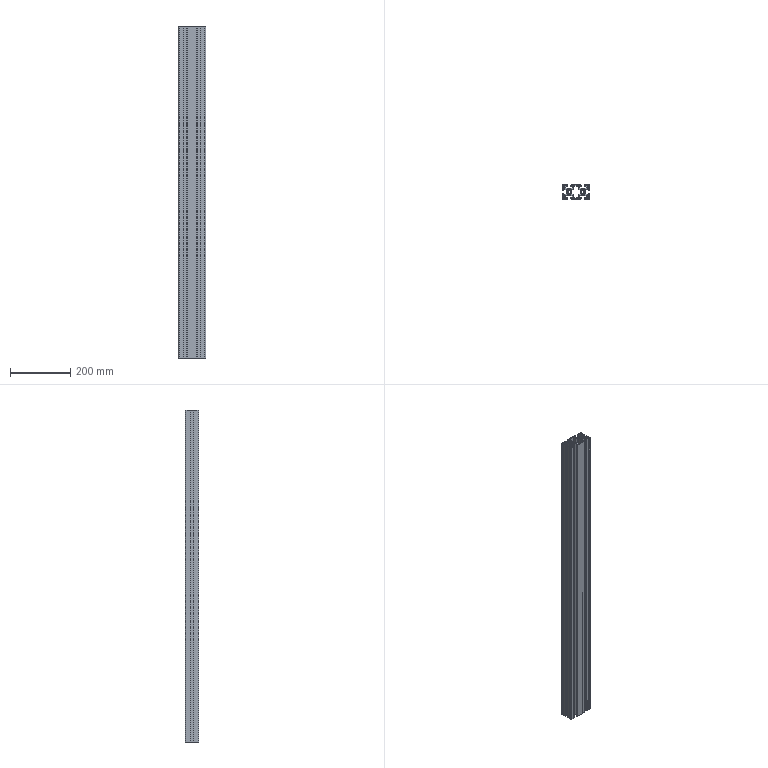Part | STEP file | OB4590-L3 | 1 solid | 256 faces | box 90 x 45 x 1100 mm | volume 1405865 mm3 | plane 174 | cylinder 82 | commonest cylinder face diameters 1 x24 2 x20 10.2 x18 16 x16 5 x4